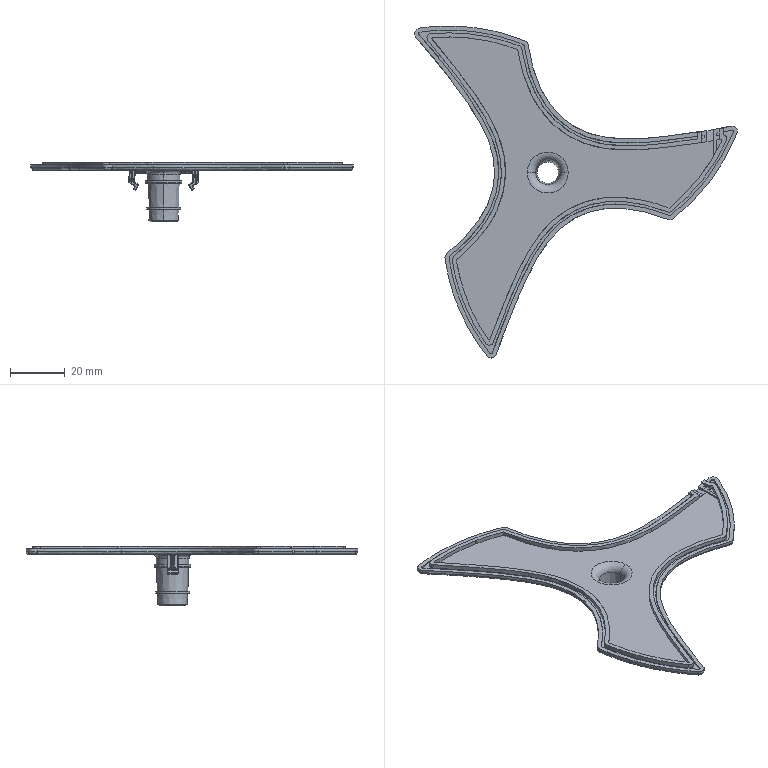Part | STEP file | ZXCOMPANY_A722-L-148 | 1 solid | 351 faces | box 117.864 x 121.275 x 21.8 mm | volume 9245 mm3 | cylinder 140 | plane 65 | spline 53 | other 32 | torus 29 | sphere 20 | cone 12 | commonest cylinder face diameters 0.6 x80 0.4 x8 3 x6 1 x5 140.86 x5 143.86 x5